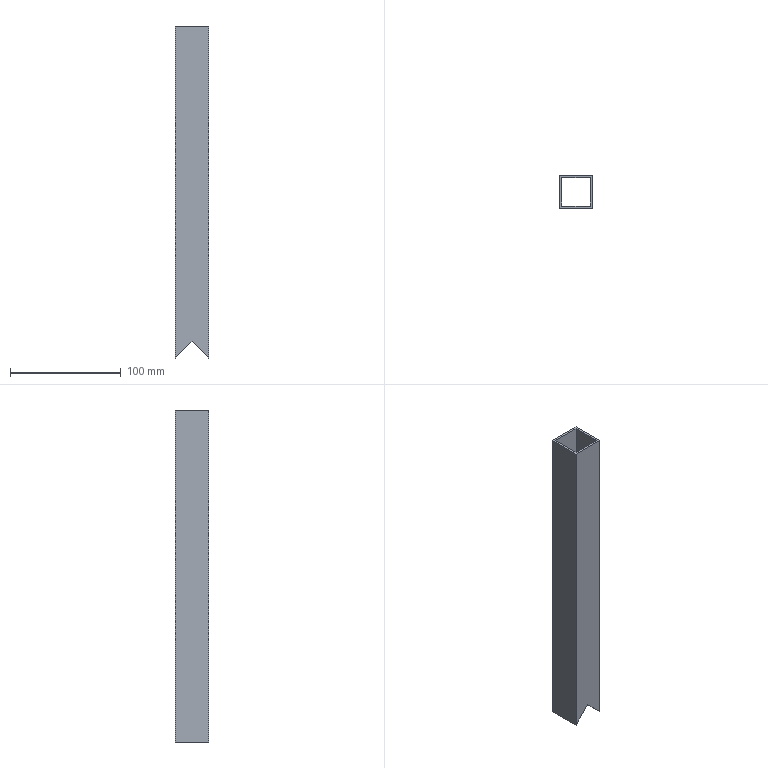Part | SolidWorks | features Extrusion 1, ICE 1 | 1 solid | 11 faces | box 30 x 30 x 300 mm | volume 66196 mm3 | plane 11
STEP:
#1=CARTESIAN_POINT('',(-15.,15.,150.));
#2=VERTEX_POINT('',#1);
#3=CARTESIAN_POINT('',(-15.,-15.,150.));
#4=VERTEX_POINT('',#3);
#5=CARTESIAN_POINT('',(-15.,-15.,150.));
#6=DIRECTION('',(0.,-1.,0.));
#7=VECTOR('',#6,1000.);
#8=LINE('',#5,#7);
#9=EDGE_CURVE('',#2,#4,#8,.T.);
#10=ORIENTED_EDGE('',*,*,#9,.T.);
#11=CARTESIAN_POINT('',(15.,-15.,150.));
#12=VERTEX_POINT('',#11);
#13=CARTESIAN_POINT('',(15.,-15.,150.));
#14=DIRECTION('',(1.,0.,0.));
#15=VECTOR('',#14,1000.);
#16=LINE('',#13,#15);
#17=EDGE_CURVE('',#4,#12,#16,.T.);
#18=ORIENTED_EDGE('',*,*,#17,.T.);
#19=CARTESIAN_POINT('',(15.,15.,150.));
#20=VERTEX_POINT('',#19);
#21=CARTESIAN_POINT('',(15.,-15.,150.));
#22=DIRECTION('',(0.,1.,0.));
#23=VECTOR('',#22,1000.);
#24=LINE('',#21,#23);
#25=EDGE_CURVE('',#12,#20,#24,.T.);
#26=ORIENTED_EDGE('',*,*,#25,.T.);
#27=CARTESIAN_POINT('',(15.,15.,150.));
#28=DIRECTION('',(-1.,0.,0.));
#29=VECTOR('',#28,1000.);
#30=LINE('',#27,#29);
#31=EDGE_CURVE('',#20,#2,#30,.T.);
#32=ORIENTED_EDGE('',*,*,#31,.T.);
#33=EDGE_LOOP('',(#10,#18,#26,#32));
#34=FACE_OUTER_BOUND('',#33,.T.);
#35=CARTESIAN_POINT('',(13.,-13.,150.));
#36=VERTEX_POINT('',#35);
#37=CARTESIAN_POINT('',(13.,13.,150.));
#38=VERTEX_POINT('',#37);
#39=CARTESIAN_POINT('',(13.,-13.,150.));
#40=DIRECTION('',(0.,1.,0.));
#41=VECTOR('',#40,1000.);
#42=LINE('',#39,#41);
#43=EDGE_CURVE('',#36,#38,#42,.T.);
#44=ORIENTED_EDGE('',*,*,#43,.F.);
#45=CARTESIAN_POINT('',(-13.,-13.,150.));
#46=VERTEX_POINT('',#45);
#47=CARTESIAN_POINT('',(13.,-13.,150.));
#48=DIRECTION('',(1.,0.,0.));
#49=VECTOR('',#48,1000.);
#50=LINE('',#47,#49);
#51=EDGE_CURVE('',#46,#36,#50,.T.);
#52=ORIENTED_EDGE('',*,*,#51,.F.);
#53=CARTESIAN_POINT('',(-13.,13.,150.));
#54=VERTEX_POINT('',#53);
#55=CARTESIAN_POINT('',(-13.,-13.,150.));
#56=DIRECTION('',(0.,-1.,0.));
#57=VECTOR('',#56,1000.);
#58=LINE('',#55,#57);
#59=EDGE_CURVE('',#54,#46,#58,.T.);
#60=ORIENTED_EDGE('',*,*,#59,.F.);
#61=CARTESIAN_POINT('',(13.,13.,150.));
#62=DIRECTION('',(-1.,0.,0.));
#63=VECTOR('',#62,1000.);
#64=LINE('',#61,#63);
#65=EDGE_CURVE('',#38,#54,#64,.T.);
#66=ORIENTED_EDGE('',*,*,#65,.F.);
#67=EDGE_LOOP('',(#44,#52,#60,#66));
#68=FACE_BOUND('',#67,.T.);
#69=CARTESIAN_POINT('',(0.,0.,150.));
#70=DIRECTION('',(0.,0.,1.));
#71=DIRECTION('',(1.,0.,0.));
#72=AXIS2_PLACEMENT_3D('',#69,#70,#71);
#73=PLANE('',#72);
#74=ADVANCED_FACE('',(#34,#68),#73,.T.);
#75=CARTESIAN_POINT('',(-15.,15.,-150.));
#76=VERTEX_POINT('',#75);
#77=CARTESIAN_POINT('',(-15.,-15.,-150.));
#78=VERTEX_POINT('',#77);
#79=CARTESIAN_POINT('',(-15.,-15.,-150.));
#80=DIRECTION('',(0.,-1.,0.));
#81=VECTOR('',#80,1000.);
#82=LINE('',#79,#81);
#83=EDGE_CURVE('',#76,#78,#82,.T.);
#84=ORIENTED_EDGE('',*,*,#83,.T.);
#85=CARTESIAN_POINT('',(-15.,-15.,150.));
#86=DIRECTION('',(0.,0.,-1.));
#87=VECTOR('',#86,1000.);
#88=LINE('',#85,#87);
#89=EDGE_CURVE('',#4,#78,#88,.T.);
#90=ORIENTED_EDGE('',*,*,#89,.F.);
#91=ORIENTED_EDGE('',*,*,#9,.F.);
#92=CARTESIAN_POINT('',(-15.,15.,150.));
#93=DIRECTION('',(0.,0.,-1.));
#94=VECTOR('',#93,1000.);
#95=LINE('',#92,#94);
#96=EDGE_CURVE('',#2,#76,#95,.T.);
#97=ORIENTED_EDGE('',*,*,#96,.T.);
#98=EDGE_LOOP('',(#84,#90,#91,#97));
#99=FACE_OUTER_BOUND('',#98,.T.);
#100=CARTESIAN_POINT('',(-15.,-15.,150.));
#101=DIRECTION('',(1.,0.,0.));
#102=DIRECTION('',(0.,1.,0.));
#103=AXIS2_PLACEMENT_3D('',#100,#101,#102);
#104=PLANE('',#103);
#105=ADVANCED_FACE('',(#99),#104,.F.);
#106=CARTESIAN_POINT('',(0.,-15.,-135.));
#107=VERTEX_POINT('',#106);
#108=CARTESIAN_POINT('',(150.,-15.,15.));
#109=DIRECTION('',(0.7071,0.,0.7071));
#110=VECTOR('',#109,1000.);
#111=LINE('',#108,#110);
#112=EDGE_CURVE('',#78,#107,#111,.T.);
#113=ORIENTED_EDGE('',*,*,#112,.T.);
#114=CARTESIAN_POINT('',(15.,-15.,-150.));
#115=VERTEX_POINT('',#114);
#116=CARTESIAN_POINT('',(-135.,-15.,0.));
#117=DIRECTION('',(0.7071,0.,-0.7071));
#118=VECTOR('',#117,1000.);
#119=LINE('',#116,#118);
#120=EDGE_CURVE('',#107,#115,#119,.T.);
#121=ORIENTED_EDGE('',*,*,#120,.T.);
#122=CARTESIAN_POINT('',(15.,-15.,150.));
#123=DIRECTION('',(0.,0.,-1.));
#124=VECTOR('',#123,1000.);
#125=LINE('',#122,#124);
#126=EDGE_CURVE('',#12,#115,#125,.T.);
#127=ORIENTED_EDGE('',*,*,#126,.F.);
#128=ORIENTED_EDGE('',*,*,#17,.F.);
#129=ORIENTED_EDGE('',*,*,#89,.T.);
#130=EDGE_LOOP('',(#113,#121,#127,#128,#129));
#131=FACE_OUTER_BOUND('',#130,.T.);
#132=CARTESIAN_POINT('',(15.,-15.,150.));
#133=DIRECTION('',(0.,1.,0.));
#134=DIRECTION('',(-1.,0.,0.));
#135=AXIS2_PLACEMENT_3D('',#132,#133,#134);
#136=PLANE('',#135);
#137=ADVANCED_FACE('',(#131),#136,.F.);
#138=CARTESIAN_POINT('',(15.,15.,-150.));
#139=VERTEX_POINT('',#138);
#140=CARTESIAN_POINT('',(15.,-15.,-150.));
#141=DIRECTION('',(0.,1.,0.));
#142=VECTOR('',#141,1000.);
#143=LINE('',#140,#142);
#144=EDGE_CURVE('',#115,#139,#143,.T.);
#145=ORIENTED_EDGE('',*,*,#144,.T.);
#146=CARTESIAN_POINT('',(15.,15.,150.));
#147=DIRECTION('',(0.,0.,-1.));
#148=VECTOR('',#147,1000.);
#149=LINE('',#146,#148);
#150=EDGE_CURVE('',#20,#139,#149,.T.);
#151=ORIENTED_EDGE('',*,*,#150,.F.);
#152=ORIENTED_EDGE('',*,*,#25,.F.);
#153=ORIENTED_EDGE('',*,*,#126,.T.);
#154=EDGE_LOOP('',(#145,#151,#152,#153));
#155=FACE_OUTER_BOUND('',#154,.T.);
#156=CARTESIAN_POINT('',(15.,-15.,150.));
#157=DIRECTION('',(-1.,0.,0.));
#158=DIRECTION('',(0.,0.,1.));
#159=AXIS2_PLACEMENT_3D('',#156,#157,#158);
#160=PLANE('',#159);
#161=ADVANCED_FACE('',(#155),#160,.F.);
#162=ORIENTED_EDGE('',*,*,#150,.T.);
#163=CARTESIAN_POINT('',(0.,15.,-135.));
#164=VERTEX_POINT('',#163);
#165=CARTESIAN_POINT('',(0.,15.,-135.));
#166=DIRECTION('',(0.7071,0.,-0.7071));
#167=VECTOR('',#166,1000.);
#168=LINE('',#165,#167);
#169=EDGE_CURVE('',#164,#139,#168,.T.);
#170=ORIENTED_EDGE('',*,*,#169,.F.);
#171=CARTESIAN_POINT('',(-15.,15.,-150.));
#172=DIRECTION('',(0.7071,0.,0.7071));
#173=VECTOR('',#172,1000.);
#174=LINE('',#171,#173);
#175=EDGE_CURVE('',#76,#164,#174,.T.);
#176=ORIENTED_EDGE('',*,*,#175,.F.);
#177=ORIENTED_EDGE('',*,*,#96,.F.);
#178=ORIENTED_EDGE('',*,*,#31,.F.);
#179=EDGE_LOOP('',(#162,#170,#176,#177,#178));
#180=FACE_OUTER_BOUND('',#179,.T.);
#181=CARTESIAN_POINT('',(15.,15.,150.));
#182=DIRECTION('',(0.,-1.,0.));
#183=DIRECTION('',(0.,0.,-1.));
#184=AXIS2_PLACEMENT_3D('',#181,#182,#183);
#185=PLANE('',#184);
#186=ADVANCED_FACE('',(#180),#185,.F.);
#187=CARTESIAN_POINT('',(0.,-13.,-135.));
#188=VERTEX_POINT('',#187);
#189=CARTESIAN_POINT('',(13.,-13.,-148.));
#190=VERTEX_POINT('',#189);
#191=CARTESIAN_POINT('',(-136.,-13.,1.));
#192=DIRECTION('',(0.7071,0.,-0.7071));
#193=VECTOR('',#192,1000.);
#194=LINE('',#191,#193);
#195=EDGE_CURVE('',#188,#190,#194,.T.);
#196=ORIENTED_EDGE('',*,*,#195,.F.);
#197=CARTESIAN_POINT('',(-13.,-13.,-148.));
#198=VERTEX_POINT('',#197);
#199=CARTESIAN_POINT('',(149.,-13.,14.));
#200=DIRECTION('',(0.7071,0.,0.7071));
#201=VECTOR('',#200,1000.);
#202=LINE('',#199,#201);
#203=EDGE_CURVE('',#198,#188,#202,.T.);
#204=ORIENTED_EDGE('',*,*,#203,.F.);
#205=CARTESIAN_POINT('',(-13.,-13.,150.));
#206=DIRECTION('',(0.,0.,-1.));
#207=VECTOR('',#206,1000.);
#208=LINE('',#205,#207);
#209=EDGE_CURVE('',#46,#198,#208,.T.);
#210=ORIENTED_EDGE('',*,*,#209,.F.);
#211=ORIENTED_EDGE('',*,*,#51,.T.);
#212=CARTESIAN_POINT('',(13.,-13.,150.));
#213=DIRECTION('',(0.,0.,-1.));
#214=VECTOR('',#213,1000.);
#215=LINE('',#212,#214);
#216=EDGE_CURVE('',#36,#190,#215,.T.);
#217=ORIENTED_EDGE('',*,*,#216,.T.);
#218=EDGE_LOOP('',(#196,#204,#210,#211,#217));
#219=FACE_OUTER_BOUND('',#218,.T.);
#220=CARTESIAN_POINT('',(13.,-13.,150.));
#221=DIRECTION('',(0.,1.,0.));
#222=DIRECTION('',(0.,0.,1.));
#223=AXIS2_PLACEMENT_3D('',#220,#221,#222);
#224=PLANE('',#223);
#225=ADVANCED_FACE('',(#219),#224,.T.);
#226=CARTESIAN_POINT('',(13.,13.,-148.));
#227=VERTEX_POINT('',#226);
#228=CARTESIAN_POINT('',(13.,-13.,-148.));
#229=DIRECTION('',(0.,1.,0.));
#230=VECTOR('',#229,1000.);
#231=LINE('',#228,#230);
#232=EDGE_CURVE('',#190,#227,#231,.T.);
#233=ORIENTED_EDGE('',*,*,#232,.F.);
#234=ORIENTED_EDGE('',*,*,#216,.F.);
#235=ORIENTED_EDGE('',*,*,#43,.T.);
#236=CARTESIAN_POINT('',(13.,13.,150.));
#237=DIRECTION('',(0.,0.,-1.));
#238=VECTOR('',#237,1000.);
#239=LINE('',#236,#238);
#240=EDGE_CURVE('',#38,#227,#239,.T.);
#241=ORIENTED_EDGE('',*,*,#240,.T.);
#242=EDGE_LOOP('',(#233,#234,#235,#241));
#243=FACE_OUTER_BOUND('',#242,.T.);
#244=CARTESIAN_POINT('',(13.,-13.,150.));
#245=DIRECTION('',(-1.,0.,0.));
#246=DIRECTION('',(0.,0.,1.));
#247=AXIS2_PLACEMENT_3D('',#244,#245,#246);
#248=PLANE('',#247);
#249=ADVANCED_FACE('',(#243),#248,.T.);
#250=CARTESIAN_POINT('',(0.,13.,-135.));
#251=VERTEX_POINT('',#250);
#252=CARTESIAN_POINT('',(-136.,13.,1.));
#253=DIRECTION('',(-0.7071,0.,0.7071));
#254=VECTOR('',#253,1000.);
#255=LINE('',#252,#254);
#256=EDGE_CURVE('',#227,#251,#255,.T.);
#257=ORIENTED_EDGE('',*,*,#256,.F.);
#258=ORIENTED_EDGE('',*,*,#240,.F.);
#259=ORIENTED_EDGE('',*,*,#65,.T.);
#260=CARTESIAN_POINT('',(-13.,13.,-148.));
#261=VERTEX_POINT('',#260);
#262=CARTESIAN_POINT('',(-13.,13.,150.));
#263=DIRECTION('',(0.,0.,-1.));
#264=VECTOR('',#263,1000.);
#265=LINE('',#262,#264);
#266=EDGE_CURVE('',#54,#261,#265,.T.);
#267=ORIENTED_EDGE('',*,*,#266,.T.);
#268=CARTESIAN_POINT('',(149.,13.,14.));
#269=DIRECTION('',(-0.7071,0.,-0.7071));
#270=VECTOR('',#269,1000.);
#271=LINE('',#268,#270);
#272=EDGE_CURVE('',#251,#261,#271,.T.);
#273=ORIENTED_EDGE('',*,*,#272,.F.);
#274=EDGE_LOOP('',(#257,#258,#259,#267,#273));
#275=FACE_OUTER_BOUND('',#274,.T.);
#276=CARTESIAN_POINT('',(13.,13.,150.));
#277=DIRECTION('',(0.,-1.,0.));
#278=DIRECTION('',(0.,0.,-1.));
#279=AXIS2_PLACEMENT_3D('',#276,#277,#278);
#280=PLANE('',#279);
#281=ADVANCED_FACE('',(#275),#280,.T.);
#282=CARTESIAN_POINT('',(-13.,-13.,-148.));
#283=DIRECTION('',(0.,-1.,0.));
#284=VECTOR('',#283,1000.);
#285=LINE('',#282,#284);
#286=EDGE_CURVE('',#261,#198,#285,.T.);
#287=ORIENTED_EDGE('',*,*,#286,.F.);
#288=ORIENTED_EDGE('',*,*,#266,.F.);
#289=ORIENTED_EDGE('',*,*,#59,.T.);
#290=ORIENTED_EDGE('',*,*,#209,.T.);
#291=EDGE_LOOP('',(#287,#288,#289,#290));
#292=FACE_OUTER_BOUND('',#291,.T.);
#293=CARTESIAN_POINT('',(-13.,-13.,150.));
#294=DIRECTION('',(1.,0.,0.));
#295=DIRECTION('',(0.,0.,-1.));
#296=AXIS2_PLACEMENT_3D('',#293,#294,#295);
#297=PLANE('',#296);
#298=ADVANCED_FACE('',(#292),#297,.T.);
#299=CARTESIAN_POINT('',(0.,-87.,-135.));
#300=DIRECTION('',(0.,1.,0.));
#301=VECTOR('',#300,1000.);
#302=LINE('',#299,#301);
#303=EDGE_CURVE('',#107,#188,#302,.T.);
#304=ORIENTED_EDGE('',*,*,#303,.T.);
#305=ORIENTED_EDGE('',*,*,#195,.T.);
#306=ORIENTED_EDGE('',*,*,#232,.T.);
#307=ORIENTED_EDGE('',*,*,#256,.T.);
#308=CARTESIAN_POINT('',(0.,-87.,-135.));
#309=DIRECTION('',(0.,1.,0.));
#310=VECTOR('',#309,1000.);
#311=LINE('',#308,#310);
#312=EDGE_CURVE('',#251,#164,#311,.T.);
#313=ORIENTED_EDGE('',*,*,#312,.T.);
#314=ORIENTED_EDGE('',*,*,#169,.T.);
#315=ORIENTED_EDGE('',*,*,#144,.F.);
#316=ORIENTED_EDGE('',*,*,#120,.F.);
#317=EDGE_LOOP('',(#304,#305,#306,#307,#313,#314,#315,#316));
#318=FACE_OUTER_BOUND('',#317,.T.);
#319=CARTESIAN_POINT('',(0.,-87.,-135.));
#320=DIRECTION('',(0.7071,0.,0.7071));
#321=DIRECTION('',(0.7071,0.,-0.7071));
#322=AXIS2_PLACEMENT_3D('',#319,#320,#321);
#323=PLANE('',#322);
#324=ADVANCED_FACE('',(#318),#323,.F.);
#325=ORIENTED_EDGE('',*,*,#83,.F.);
#326=ORIENTED_EDGE('',*,*,#175,.T.);
#327=ORIENTED_EDGE('',*,*,#312,.F.);
#328=ORIENTED_EDGE('',*,*,#272,.T.);
#329=ORIENTED_EDGE('',*,*,#286,.T.);
#330=ORIENTED_EDGE('',*,*,#203,.T.);
#331=ORIENTED_EDGE('',*,*,#303,.F.);
#332=ORIENTED_EDGE('',*,*,#112,.F.);
#333=EDGE_LOOP('',(#325,#326,#327,#328,#329,#330,#331,#332));
#334=FACE_OUTER_BOUND('',#333,.T.);
#335=CARTESIAN_POINT('',(-15.,-87.,-150.));
#336=DIRECTION('',(-0.7071,0.,0.7071));
#337=DIRECTION('',(0.7071,0.,0.7071));
#338=AXIS2_PLACEMENT_3D('',#335,#336,#337);
#339=PLANE('',#338);
#340=ADVANCED_FACE('',(#334),#339,.F.);
#341=CLOSED_SHELL('',(#74,#105,#137,#161,#186,#225,#249,#281,#298,#324,#340));
#342=MANIFOLD_SOLID_BREP('',#341);
#343=CARTESIAN_POINT('',(0.,0.,0.));
#344=DIRECTION('',(0.,0.,1.));
#345=DIRECTION('',(1.,0.,0.));
#346=AXIS2_PLACEMENT_3D('',#343,#344,#345);
#347=(LENGTH_UNIT()NAMED_UNIT(*)SI_UNIT(.MILLI.,.METRE.));
#348=UNCERTAINTY_MEASURE_WITH_UNIT(LENGTH_MEASURE(0.00001),#347,'','');
#349=(NAMED_UNIT(*)PLANE_ANGLE_UNIT()SI_UNIT($,.RADIAN.));
#350=(NAMED_UNIT(*)SI_UNIT($,.STERADIAN.)SOLID_ANGLE_UNIT());
#351=(GEOMETRIC_REPRESENTATION_CONTEXT(3)GLOBAL_UNCERTAINTY_ASSIGNED_CONTEXT((#348))GLOBAL_UNIT_ASSIGNED_CONTEXT((#347,#349,#350))REPRESENTATION_CONTEXT('',''));
#352=ADVANCED_BREP_SHAPE_REPRESENTATION('',(#342,#346),#351);